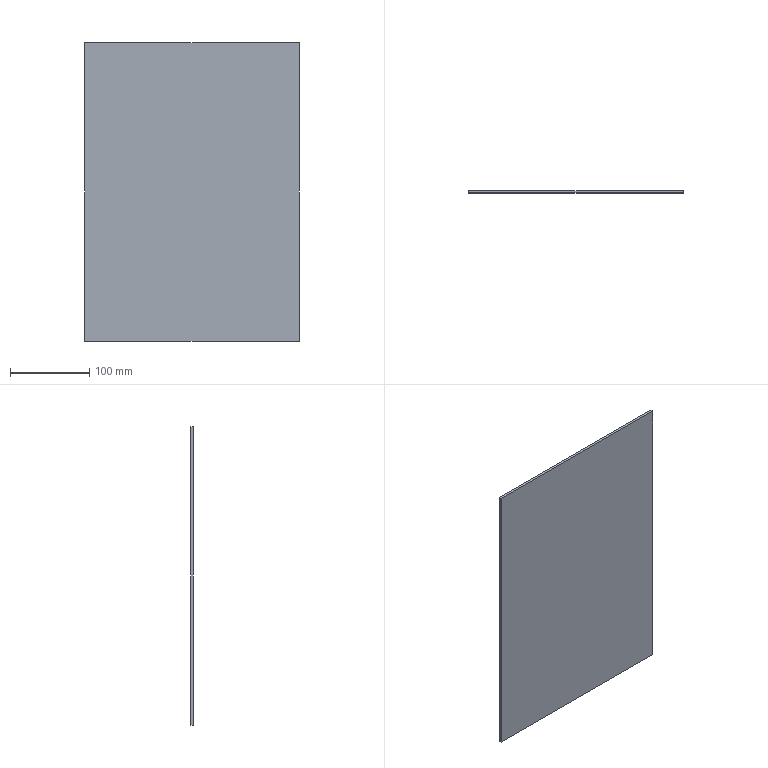Part | SolidWorks | features FlatPattern 1, SMBaseFlange 1, SheetMetal 1 | 1 solid | 6 faces | box 270 x 3 x 376 mm | volume 304560 mm3 | plane 6
STEP:
#1=CARTESIAN_POINT('',(135.,0.,188.));
#2=VERTEX_POINT('',#1);
#3=CARTESIAN_POINT('',(135.,0.,-188.));
#4=VERTEX_POINT('',#3);
#5=CARTESIAN_POINT('',(135.,0.,-188.));
#6=DIRECTION('',(0.,0.,-1.));
#7=VECTOR('',#6,1000.);
#8=LINE('',#5,#7);
#9=EDGE_CURVE('',#2,#4,#8,.T.);
#10=ORIENTED_EDGE('',*,*,#9,.T.);
#11=CARTESIAN_POINT('',(135.,3.,-188.));
#12=VERTEX_POINT('',#11);
#13=CARTESIAN_POINT('',(135.,3.,-188.));
#14=DIRECTION('',(0.,-1.,0.));
#15=VECTOR('',#14,1000.);
#16=LINE('',#13,#15);
#17=EDGE_CURVE('',#12,#4,#16,.T.);
#18=ORIENTED_EDGE('',*,*,#17,.F.);
#19=CARTESIAN_POINT('',(135.,3.,188.));
#20=VERTEX_POINT('',#19);
#21=CARTESIAN_POINT('',(135.,3.,-188.));
#22=DIRECTION('',(0.,0.,-1.));
#23=VECTOR('',#22,1000.);
#24=LINE('',#21,#23);
#25=EDGE_CURVE('',#20,#12,#24,.T.);
#26=ORIENTED_EDGE('',*,*,#25,.F.);
#27=CARTESIAN_POINT('',(135.,3.,188.));
#28=DIRECTION('',(0.,-1.,0.));
#29=VECTOR('',#28,1000.);
#30=LINE('',#27,#29);
#31=EDGE_CURVE('',#20,#2,#30,.T.);
#32=ORIENTED_EDGE('',*,*,#31,.T.);
#33=EDGE_LOOP('',(#10,#18,#26,#32));
#34=FACE_OUTER_BOUND('',#33,.T.);
#35=CARTESIAN_POINT('',(135.,3.,-188.));
#36=DIRECTION('',(-1.,0.,0.));
#37=DIRECTION('',(0.,0.,1.));
#38=AXIS2_PLACEMENT_3D('',#35,#36,#37);
#39=PLANE('',#38);
#40=ADVANCED_FACE('',(#34),#39,.F.);
#41=CARTESIAN_POINT('',(-135.,0.,-188.));
#42=VERTEX_POINT('',#41);
#43=CARTESIAN_POINT('',(-135.,0.,-188.));
#44=DIRECTION('',(-1.,0.,0.));
#45=VECTOR('',#44,1000.);
#46=LINE('',#43,#45);
#47=EDGE_CURVE('',#4,#42,#46,.T.);
#48=ORIENTED_EDGE('',*,*,#47,.T.);
#49=CARTESIAN_POINT('',(-135.,3.,-188.));
#50=VERTEX_POINT('',#49);
#51=CARTESIAN_POINT('',(-135.,3.,-188.));
#52=DIRECTION('',(0.,-1.,0.));
#53=VECTOR('',#52,1000.);
#54=LINE('',#51,#53);
#55=EDGE_CURVE('',#50,#42,#54,.T.);
#56=ORIENTED_EDGE('',*,*,#55,.F.);
#57=CARTESIAN_POINT('',(-135.,3.,-188.));
#58=DIRECTION('',(-1.,0.,0.));
#59=VECTOR('',#58,1000.);
#60=LINE('',#57,#59);
#61=EDGE_CURVE('',#12,#50,#60,.T.);
#62=ORIENTED_EDGE('',*,*,#61,.F.);
#63=ORIENTED_EDGE('',*,*,#17,.T.);
#64=EDGE_LOOP('',(#48,#56,#62,#63));
#65=FACE_OUTER_BOUND('',#64,.T.);
#66=CARTESIAN_POINT('',(-135.,3.,-188.));
#67=DIRECTION('',(0.,0.,1.));
#68=DIRECTION('',(1.,0.,0.));
#69=AXIS2_PLACEMENT_3D('',#66,#67,#68);
#70=PLANE('',#69);
#71=ADVANCED_FACE('',(#65),#70,.F.);
#72=CARTESIAN_POINT('',(-135.,0.,188.));
#73=VERTEX_POINT('',#72);
#74=CARTESIAN_POINT('',(-135.,0.,-188.));
#75=DIRECTION('',(0.,0.,1.));
#76=VECTOR('',#75,1000.);
#77=LINE('',#74,#76);
#78=EDGE_CURVE('',#42,#73,#77,.T.);
#79=ORIENTED_EDGE('',*,*,#78,.T.);
#80=CARTESIAN_POINT('',(-135.,3.,188.));
#81=VERTEX_POINT('',#80);
#82=CARTESIAN_POINT('',(-135.,3.,188.));
#83=DIRECTION('',(0.,-1.,0.));
#84=VECTOR('',#83,1000.);
#85=LINE('',#82,#84);
#86=EDGE_CURVE('',#81,#73,#85,.T.);
#87=ORIENTED_EDGE('',*,*,#86,.F.);
#88=CARTESIAN_POINT('',(-135.,3.,-188.));
#89=DIRECTION('',(0.,0.,1.));
#90=VECTOR('',#89,1000.);
#91=LINE('',#88,#90);
#92=EDGE_CURVE('',#50,#81,#91,.T.);
#93=ORIENTED_EDGE('',*,*,#92,.F.);
#94=ORIENTED_EDGE('',*,*,#55,.T.);
#95=EDGE_LOOP('',(#79,#87,#93,#94));
#96=FACE_OUTER_BOUND('',#95,.T.);
#97=CARTESIAN_POINT('',(-135.,3.,-188.));
#98=DIRECTION('',(1.,0.,0.));
#99=DIRECTION('',(0.,0.,-1.));
#100=AXIS2_PLACEMENT_3D('',#97,#98,#99);
#101=PLANE('',#100);
#102=ADVANCED_FACE('',(#96),#101,.F.);
#103=CARTESIAN_POINT('',(-135.,0.,188.));
#104=DIRECTION('',(1.,0.,0.));
#105=VECTOR('',#104,1000.);
#106=LINE('',#103,#105);
#107=EDGE_CURVE('',#73,#2,#106,.T.);
#108=ORIENTED_EDGE('',*,*,#107,.T.);
#109=ORIENTED_EDGE('',*,*,#31,.F.);
#110=CARTESIAN_POINT('',(-135.,3.,188.));
#111=DIRECTION('',(1.,0.,0.));
#112=VECTOR('',#111,1000.);
#113=LINE('',#110,#112);
#114=EDGE_CURVE('',#81,#20,#113,.T.);
#115=ORIENTED_EDGE('',*,*,#114,.F.);
#116=ORIENTED_EDGE('',*,*,#86,.T.);
#117=EDGE_LOOP('',(#108,#109,#115,#116));
#118=FACE_OUTER_BOUND('',#117,.T.);
#119=CARTESIAN_POINT('',(-135.,3.,188.));
#120=DIRECTION('',(0.,0.,-1.));
#121=DIRECTION('',(-1.,0.,0.));
#122=AXIS2_PLACEMENT_3D('',#119,#120,#121);
#123=PLANE('',#122);
#124=ADVANCED_FACE('',(#118),#123,.F.);
#125=ORIENTED_EDGE('',*,*,#25,.T.);
#126=ORIENTED_EDGE('',*,*,#61,.T.);
#127=ORIENTED_EDGE('',*,*,#92,.T.);
#128=ORIENTED_EDGE('',*,*,#114,.T.);
#129=EDGE_LOOP('',(#125,#126,#127,#128));
#130=FACE_OUTER_BOUND('',#129,.T.);
#131=CARTESIAN_POINT('',(0.,3.,0.));
#132=DIRECTION('',(0.,1.,0.));
#133=DIRECTION('',(0.,0.,1.));
#134=AXIS2_PLACEMENT_3D('',#131,#132,#133);
#135=PLANE('',#134);
#136=ADVANCED_FACE('',(#130),#135,.T.);
#137=ORIENTED_EDGE('',*,*,#9,.F.);
#138=ORIENTED_EDGE('',*,*,#107,.F.);
#139=ORIENTED_EDGE('',*,*,#78,.F.);
#140=ORIENTED_EDGE('',*,*,#47,.F.);
#141=EDGE_LOOP('',(#137,#138,#139,#140));
#142=FACE_OUTER_BOUND('',#141,.T.);
#143=CARTESIAN_POINT('',(0.,0.,0.));
#144=DIRECTION('',(0.,1.,0.));
#145=DIRECTION('',(0.,0.,1.));
#146=AXIS2_PLACEMENT_3D('',#143,#144,#145);
#147=PLANE('',#146);
#148=ADVANCED_FACE('',(#142),#147,.F.);
#149=CLOSED_SHELL('',(#40,#71,#102,#124,#136,#148));
#150=MANIFOLD_SOLID_BREP('',#149);
#151=CARTESIAN_POINT('',(0.,0.,0.));
#152=DIRECTION('',(0.,0.,1.));
#153=DIRECTION('',(1.,0.,0.));
#154=AXIS2_PLACEMENT_3D('',#151,#152,#153);
#155=(LENGTH_UNIT()NAMED_UNIT(*)SI_UNIT(.MILLI.,.METRE.));
#156=UNCERTAINTY_MEASURE_WITH_UNIT(LENGTH_MEASURE(0.00001),#155,'','');
#157=(NAMED_UNIT(*)PLANE_ANGLE_UNIT()SI_UNIT($,.RADIAN.));
#158=(NAMED_UNIT(*)SI_UNIT($,.STERADIAN.)SOLID_ANGLE_UNIT());
#159=(GEOMETRIC_REPRESENTATION_CONTEXT(3)GLOBAL_UNCERTAINTY_ASSIGNED_CONTEXT((#156))GLOBAL_UNIT_ASSIGNED_CONTEXT((#155,#157,#158))REPRESENTATION_CONTEXT('',''));
#160=ADVANCED_BREP_SHAPE_REPRESENTATION('',(#150,#154),#159);